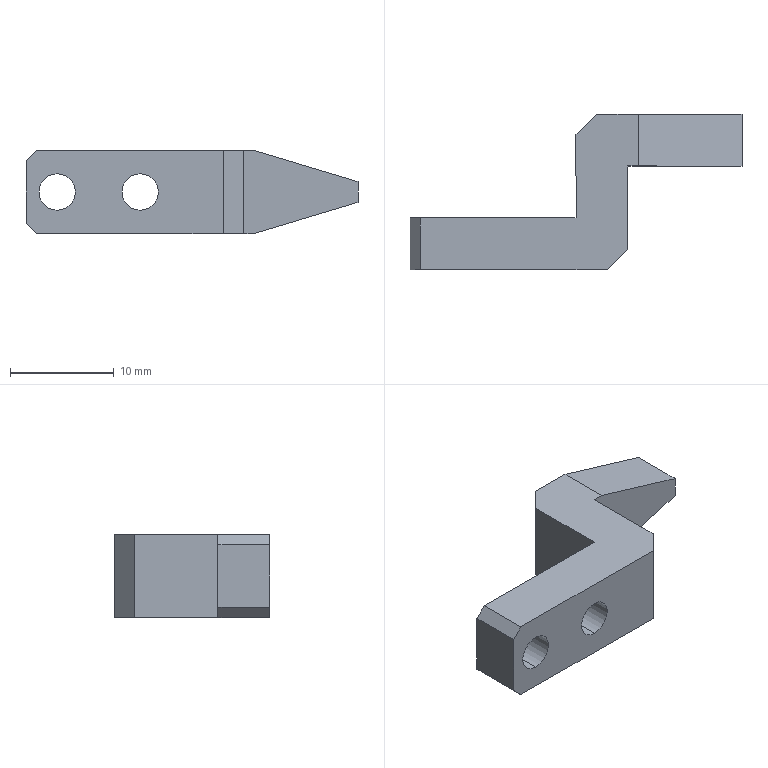Part | SolidWorks | features Chamfer 4, Extrusion 1, HoleWzd 1, ICE 1 | 1 solid | 20 faces | box 32 x 15 x 8 mm | volume 1397 mm3 | plane 16 | cylinder 4 | commonest cylinder face diameters 3.5 x4
STEP:
#1=CARTESIAN_POINT('',(-13.,-7.5,-1.75));
#2=VERTEX_POINT('',#1);
#3=CARTESIAN_POINT('',(-13.,-7.5,1.75));
#4=VERTEX_POINT('',#3);
#5=CARTESIAN_POINT('',(-13.,-7.5,0.));
#6=DIRECTION('',(0.,1.,0.));
#7=DIRECTION('',(0.,0.,1.));
#8=AXIS2_PLACEMENT_3D('',#5,#6,#7);
#9=CIRCLE('',#8,1.75);
#10=EDGE_CURVE('',#2,#4,#9,.T.);
#11=ORIENTED_EDGE('',*,*,#10,.F.);
#12=CARTESIAN_POINT('',(-13.,-2.5,-1.75));
#13=VERTEX_POINT('',#12);
#14=CARTESIAN_POINT('',(-13.,-2.5,-1.75));
#15=DIRECTION('',(0.,1.,0.));
#16=VECTOR('',#15,1000.);
#17=LINE('',#14,#16);
#18=EDGE_CURVE('',#2,#13,#17,.T.);
#19=ORIENTED_EDGE('',*,*,#18,.T.);
#20=CARTESIAN_POINT('',(-13.,-2.5,1.75));
#21=VERTEX_POINT('',#20);
#22=CARTESIAN_POINT('',(-13.,-2.5,0.));
#23=DIRECTION('',(0.,1.,0.));
#24=DIRECTION('',(0.,0.,1.));
#25=AXIS2_PLACEMENT_3D('',#22,#23,#24);
#26=CIRCLE('',#25,1.75);
#27=EDGE_CURVE('',#13,#21,#26,.T.);
#28=ORIENTED_EDGE('',*,*,#27,.T.);
#29=CARTESIAN_POINT('',(-13.,-2.5,1.75));
#30=DIRECTION('',(0.,1.,0.));
#31=VECTOR('',#30,1000.);
#32=LINE('',#29,#31);
#33=EDGE_CURVE('',#4,#21,#32,.T.);
#34=ORIENTED_EDGE('',*,*,#33,.F.);
#35=EDGE_LOOP('',(#11,#19,#28,#34));
#36=FACE_OUTER_BOUND('',#35,.T.);
#37=CARTESIAN_POINT('',(-13.,-2.5,0.));
#38=DIRECTION('',(0.,1.,0.));
#39=DIRECTION('',(0.,0.,1.));
#40=AXIS2_PLACEMENT_3D('',#37,#38,#39);
#41=CYLINDRICAL_SURFACE('',#40,1.75);
#42=ADVANCED_FACE('',(#36),#41,.F.);
#43=CARTESIAN_POINT('',(-5.,-7.5,-1.75));
#44=VERTEX_POINT('',#43);
#45=CARTESIAN_POINT('',(-5.,-7.5,1.75));
#46=VERTEX_POINT('',#45);
#47=CARTESIAN_POINT('',(-5.,-7.5,0.));
#48=DIRECTION('',(0.,1.,0.));
#49=DIRECTION('',(0.,0.,1.));
#50=AXIS2_PLACEMENT_3D('',#47,#48,#49);
#51=CIRCLE('',#50,1.75);
#52=EDGE_CURVE('',#44,#46,#51,.T.);
#53=ORIENTED_EDGE('',*,*,#52,.F.);
#54=CARTESIAN_POINT('',(-5.,-2.5,-1.75));
#55=VERTEX_POINT('',#54);
#56=CARTESIAN_POINT('',(-5.,-2.5,-1.75));
#57=DIRECTION('',(0.,1.,0.));
#58=VECTOR('',#57,1000.);
#59=LINE('',#56,#58);
#60=EDGE_CURVE('',#44,#55,#59,.T.);
#61=ORIENTED_EDGE('',*,*,#60,.T.);
#62=CARTESIAN_POINT('',(-5.,-2.5,1.75));
#63=VERTEX_POINT('',#62);
#64=CARTESIAN_POINT('',(-5.,-2.5,0.));
#65=DIRECTION('',(0.,1.,0.));
#66=DIRECTION('',(0.,0.,1.));
#67=AXIS2_PLACEMENT_3D('',#64,#65,#66);
#68=CIRCLE('',#67,1.75);
#69=EDGE_CURVE('',#55,#63,#68,.T.);
#70=ORIENTED_EDGE('',*,*,#69,.T.);
#71=CARTESIAN_POINT('',(-5.,-2.5,1.75));
#72=DIRECTION('',(0.,1.,0.));
#73=VECTOR('',#72,1000.);
#74=LINE('',#71,#73);
#75=EDGE_CURVE('',#46,#63,#74,.T.);
#76=ORIENTED_EDGE('',*,*,#75,.F.);
#77=EDGE_LOOP('',(#53,#61,#70,#76));
#78=FACE_OUTER_BOUND('',#77,.T.);
#79=CARTESIAN_POINT('',(-5.,-2.5,0.));
#80=DIRECTION('',(0.,1.,0.));
#81=DIRECTION('',(0.,0.,1.));
#82=AXIS2_PLACEMENT_3D('',#79,#80,#81);
#83=CYLINDRICAL_SURFACE('',#82,1.75);
#84=ADVANCED_FACE('',(#78),#83,.F.);
#85=CARTESIAN_POINT('',(16.,2.5,-1.));
#86=VERTEX_POINT('',#85);
#87=CARTESIAN_POINT('',(16.,2.5,1.));
#88=VERTEX_POINT('',#87);
#89=CARTESIAN_POINT('',(16.,2.5,-4.));
#90=DIRECTION('',(0.,0.,1.));
#91=VECTOR('',#90,1000.);
#92=LINE('',#89,#91);
#93=EDGE_CURVE('',#86,#88,#92,.T.);
#94=ORIENTED_EDGE('',*,*,#93,.F.);
#95=CARTESIAN_POINT('',(16.,7.5,-1.));
#96=VERTEX_POINT('',#95);
#97=CARTESIAN_POINT('',(16.,7.5,-1.));
#98=DIRECTION('',(0.,1.,0.));
#99=VECTOR('',#98,1000.);
#100=LINE('',#97,#99);
#101=EDGE_CURVE('',#86,#96,#100,.T.);
#102=ORIENTED_EDGE('',*,*,#101,.T.);
#103=CARTESIAN_POINT('',(16.,7.5,1.));
#104=VERTEX_POINT('',#103);
#105=CARTESIAN_POINT('',(16.,7.5,4.));
#106=DIRECTION('',(0.,0.,-1.));
#107=VECTOR('',#106,1000.);
#108=LINE('',#105,#107);
#109=EDGE_CURVE('',#104,#96,#108,.T.);
#110=ORIENTED_EDGE('',*,*,#109,.F.);
#111=CARTESIAN_POINT('',(16.,2.5,1.));
#112=DIRECTION('',(0.,-1.,0.));
#113=VECTOR('',#112,1000.);
#114=LINE('',#111,#113);
#115=EDGE_CURVE('',#104,#88,#114,.T.);
#116=ORIENTED_EDGE('',*,*,#115,.T.);
#117=EDGE_LOOP('',(#94,#102,#110,#116));
#118=FACE_OUTER_BOUND('',#117,.T.);
#119=CARTESIAN_POINT('',(16.,7.5,4.));
#120=DIRECTION('',(-1.,0.,0.));
#121=DIRECTION('',(0.,-1.,0.));
#122=AXIS2_PLACEMENT_3D('',#119,#120,#121);
#123=PLANE('',#122);
#124=ADVANCED_FACE('',(#118),#123,.F.);
#125=ORIENTED_EDGE('',*,*,#109,.T.);
#126=CARTESIAN_POINT('',(6.,7.5,-4.));
#127=VERTEX_POINT('',#126);
#128=CARTESIAN_POINT('',(16.,7.5,-1.));
#129=DIRECTION('',(-0.9578,0.,-0.2873));
#130=VECTOR('',#129,1000.);
#131=LINE('',#128,#130);
#132=EDGE_CURVE('',#96,#127,#131,.T.);
#133=ORIENTED_EDGE('',*,*,#132,.T.);
#134=CARTESIAN_POINT('',(2.,7.5,-4.));
#135=VERTEX_POINT('',#134);
#136=CARTESIAN_POINT('',(-16.,7.5,-4.));
#137=DIRECTION('',(-1.,0.,0.));
#138=VECTOR('',#137,1000.);
#139=LINE('',#136,#138);
#140=EDGE_CURVE('',#127,#135,#139,.T.);
#141=ORIENTED_EDGE('',*,*,#140,.T.);
#142=CARTESIAN_POINT('',(2.,7.5,4.));
#143=VERTEX_POINT('',#142);
#144=CARTESIAN_POINT('',(2.,7.5,4.));
#145=DIRECTION('',(0.,0.,1.));
#146=VECTOR('',#145,1000.);
#147=LINE('',#144,#146);
#148=EDGE_CURVE('',#135,#143,#147,.T.);
#149=ORIENTED_EDGE('',*,*,#148,.T.);
#150=CARTESIAN_POINT('',(6.,7.5,4.));
#151=VERTEX_POINT('',#150);
#152=CARTESIAN_POINT('',(-16.,7.5,4.));
#153=DIRECTION('',(-1.,0.,0.));
#154=VECTOR('',#153,1000.);
#155=LINE('',#152,#154);
#156=EDGE_CURVE('',#151,#143,#155,.T.);
#157=ORIENTED_EDGE('',*,*,#156,.F.);
#158=CARTESIAN_POINT('',(6.,7.5,4.));
#159=DIRECTION('',(0.9578,0.,-0.2873));
#160=VECTOR('',#159,1000.);
#161=LINE('',#158,#160);
#162=EDGE_CURVE('',#151,#104,#161,.T.);
#163=ORIENTED_EDGE('',*,*,#162,.T.);
#164=EDGE_LOOP('',(#125,#133,#141,#149,#157,#163));
#165=FACE_OUTER_BOUND('',#164,.T.);
#166=CARTESIAN_POINT('',(-16.,7.5,4.));
#167=DIRECTION('',(0.,-1.,0.));
#168=DIRECTION('',(0.,0.,-1.));
#169=AXIS2_PLACEMENT_3D('',#166,#167,#168);
#170=PLANE('',#169);
#171=ADVANCED_FACE('',(#165),#170,.F.);
#172=CARTESIAN_POINT('',(-16.,-2.5,-3.));
#173=VERTEX_POINT('',#172);
#174=CARTESIAN_POINT('',(-16.,-2.5,3.));
#175=VERTEX_POINT('',#174);
#176=CARTESIAN_POINT('',(-16.,-2.5,-4.));
#177=DIRECTION('',(0.,0.,1.));
#178=VECTOR('',#177,1000.);
#179=LINE('',#176,#178);
#180=EDGE_CURVE('',#173,#175,#179,.T.);
#181=ORIENTED_EDGE('',*,*,#180,.F.);
#182=CARTESIAN_POINT('',(-16.,-7.5,-3.));
#183=VERTEX_POINT('',#182);
#184=CARTESIAN_POINT('',(-16.,7.5,-3.));
#185=DIRECTION('',(0.,-1.,0.));
#186=VECTOR('',#185,1000.);
#187=LINE('',#184,#186);
#188=EDGE_CURVE('',#173,#183,#187,.T.);
#189=ORIENTED_EDGE('',*,*,#188,.T.);
#190=CARTESIAN_POINT('',(-16.,-7.5,3.));
#191=VERTEX_POINT('',#190);
#192=CARTESIAN_POINT('',(-16.,-7.5,4.));
#193=DIRECTION('',(0.,0.,-1.));
#194=VECTOR('',#193,1000.);
#195=LINE('',#192,#194);
#196=EDGE_CURVE('',#191,#183,#195,.T.);
#197=ORIENTED_EDGE('',*,*,#196,.F.);
#198=CARTESIAN_POINT('',(-16.,-2.5,3.));
#199=DIRECTION('',(0.,1.,0.));
#200=VECTOR('',#199,1000.);
#201=LINE('',#198,#200);
#202=EDGE_CURVE('',#191,#175,#201,.T.);
#203=ORIENTED_EDGE('',*,*,#202,.T.);
#204=EDGE_LOOP('',(#181,#189,#197,#203));
#205=FACE_OUTER_BOUND('',#204,.T.);
#206=CARTESIAN_POINT('',(-16.,7.5,4.));
#207=DIRECTION('',(1.,0.,0.));
#208=DIRECTION('',(0.,1.,0.));
#209=AXIS2_PLACEMENT_3D('',#206,#207,#208);
#210=PLANE('',#209);
#211=ADVANCED_FACE('',(#205),#210,.F.);
#212=CARTESIAN_POINT('',(-13.,-7.5,0.));
#213=DIRECTION('',(0.,1.,0.));
#214=DIRECTION('',(0.,0.,1.));
#215=AXIS2_PLACEMENT_3D('',#212,#213,#214);
#216=CIRCLE('',#215,1.75);
#217=EDGE_CURVE('',#4,#2,#216,.T.);
#218=ORIENTED_EDGE('',*,*,#217,.T.);
#219=ORIENTED_EDGE('',*,*,#10,.T.);
#220=EDGE_LOOP('',(#218,#219));
#221=FACE_BOUND('',#220,.T.);
#222=CARTESIAN_POINT('',(-5.,-7.5,0.));
#223=DIRECTION('',(0.,1.,0.));
#224=DIRECTION('',(0.,0.,1.));
#225=AXIS2_PLACEMENT_3D('',#222,#223,#224);
#226=CIRCLE('',#225,1.75);
#227=EDGE_CURVE('',#46,#44,#226,.T.);
#228=ORIENTED_EDGE('',*,*,#227,.T.);
#229=ORIENTED_EDGE('',*,*,#52,.T.);
#230=EDGE_LOOP('',(#228,#229));
#231=FACE_BOUND('',#230,.T.);
#232=CARTESIAN_POINT('',(-15.,-7.5,-4.));
#233=VERTEX_POINT('',#232);
#234=CARTESIAN_POINT('',(3.,-7.5,-4.));
#235=VERTEX_POINT('',#234);
#236=CARTESIAN_POINT('',(-16.,-7.5,-4.));
#237=DIRECTION('',(1.,0.,0.));
#238=VECTOR('',#237,1000.);
#239=LINE('',#236,#238);
#240=EDGE_CURVE('',#233,#235,#239,.T.);
#241=ORIENTED_EDGE('',*,*,#240,.T.);
#242=CARTESIAN_POINT('',(3.,-7.5,4.));
#243=VERTEX_POINT('',#242);
#244=CARTESIAN_POINT('',(3.,-7.5,4.));
#245=DIRECTION('',(0.,0.,1.));
#246=VECTOR('',#245,1000.);
#247=LINE('',#244,#246);
#248=EDGE_CURVE('',#235,#243,#247,.T.);
#249=ORIENTED_EDGE('',*,*,#248,.T.);
#250=CARTESIAN_POINT('',(-15.,-7.5,4.));
#251=VERTEX_POINT('',#250);
#252=CARTESIAN_POINT('',(-16.,-7.5,4.));
#253=DIRECTION('',(1.,0.,0.));
#254=VECTOR('',#253,1000.);
#255=LINE('',#252,#254);
#256=EDGE_CURVE('',#251,#243,#255,.T.);
#257=ORIENTED_EDGE('',*,*,#256,.F.);
#258=CARTESIAN_POINT('',(-15.,-7.5,4.));
#259=DIRECTION('',(-0.7071,0.,-0.7071));
#260=VECTOR('',#259,1000.);
#261=LINE('',#258,#260);
#262=EDGE_CURVE('',#251,#191,#261,.T.);
#263=ORIENTED_EDGE('',*,*,#262,.T.);
#264=ORIENTED_EDGE('',*,*,#196,.T.);
#265=CARTESIAN_POINT('',(-16.,-7.5,-3.));
#266=DIRECTION('',(0.7071,0.,-0.7071));
#267=VECTOR('',#266,1000.);
#268=LINE('',#265,#267);
#269=EDGE_CURVE('',#183,#233,#268,.T.);
#270=ORIENTED_EDGE('',*,*,#269,.T.);
#271=EDGE_LOOP('',(#241,#249,#257,#263,#264,#270));
#272=FACE_OUTER_BOUND('',#271,.T.);
#273=CARTESIAN_POINT('',(-16.,-7.5,4.));
#274=DIRECTION('',(0.,1.,0.));
#275=DIRECTION('',(0.,0.,1.));
#276=AXIS2_PLACEMENT_3D('',#273,#274,#275);
#277=PLANE('',#276);
#278=ADVANCED_FACE('',(#221,#231,#272),#277,.F.);
#279=CARTESIAN_POINT('',(6.,2.5,4.));
#280=VERTEX_POINT('',#279);
#281=CARTESIAN_POINT('',(5.,2.5,4.));
#282=VERTEX_POINT('',#281);
#283=CARTESIAN_POINT('',(16.,2.5,4.));
#284=DIRECTION('',(-1.,0.,0.));
#285=VECTOR('',#284,1000.);
#286=LINE('',#283,#285);
#287=EDGE_CURVE('',#280,#282,#286,.T.);
#288=ORIENTED_EDGE('',*,*,#287,.F.);
#289=CARTESIAN_POINT('',(6.,7.5,4.));
#290=DIRECTION('',(0.,1.,0.));
#291=VECTOR('',#290,1000.);
#292=LINE('',#289,#291);
#293=EDGE_CURVE('',#280,#151,#292,.T.);
#294=ORIENTED_EDGE('',*,*,#293,.T.);
#295=ORIENTED_EDGE('',*,*,#156,.T.);
#296=CARTESIAN_POINT('',(0.,5.5,4.));
#297=VERTEX_POINT('',#296);
#298=CARTESIAN_POINT('',(-2.75,2.75,4.));
#299=DIRECTION('',(-0.7071,-0.7071,0.));
#300=VECTOR('',#299,1000.);
#301=LINE('',#298,#300);
#302=EDGE_CURVE('',#143,#297,#301,.T.);
#303=ORIENTED_EDGE('',*,*,#302,.T.);
#304=CARTESIAN_POINT('',(0.,-2.5,4.));
#305=VERTEX_POINT('',#304);
#306=CARTESIAN_POINT('',(0.,7.5,4.));
#307=DIRECTION('',(0.,1.,0.));
#308=VECTOR('',#307,1000.);
#309=LINE('',#306,#308);
#310=EDGE_CURVE('',#305,#297,#309,.T.);
#311=ORIENTED_EDGE('',*,*,#310,.F.);
#312=CARTESIAN_POINT('',(-15.,-2.5,4.));
#313=VERTEX_POINT('',#312);
#314=CARTESIAN_POINT('',(-16.,-2.5,4.));
#315=DIRECTION('',(1.,0.,0.));
#316=VECTOR('',#315,1000.);
#317=LINE('',#314,#316);
#318=EDGE_CURVE('',#313,#305,#317,.T.);
#319=ORIENTED_EDGE('',*,*,#318,.F.);
#320=CARTESIAN_POINT('',(-15.,-7.5,4.));
#321=DIRECTION('',(0.,-1.,0.));
#322=VECTOR('',#321,1000.);
#323=LINE('',#320,#322);
#324=EDGE_CURVE('',#313,#251,#323,.T.);
#325=ORIENTED_EDGE('',*,*,#324,.T.);
#326=ORIENTED_EDGE('',*,*,#256,.T.);
#327=CARTESIAN_POINT('',(5.,-5.5,4.));
#328=VERTEX_POINT('',#327);
#329=CARTESIAN_POINT('',(5.25,-5.25,4.));
#330=DIRECTION('',(0.7071,0.7071,0.));
#331=VECTOR('',#330,1000.);
#332=LINE('',#329,#331);
#333=EDGE_CURVE('',#243,#328,#332,.T.);
#334=ORIENTED_EDGE('',*,*,#333,.T.);
#335=CARTESIAN_POINT('',(5.,-7.5,4.));
#336=DIRECTION('',(0.,-1.,0.));
#337=VECTOR('',#336,1000.);
#338=LINE('',#335,#337);
#339=EDGE_CURVE('',#282,#328,#338,.T.);
#340=ORIENTED_EDGE('',*,*,#339,.F.);
#341=EDGE_LOOP('',(#288,#294,#295,#303,#311,#319,#325,#326,#334,#340));
#342=FACE_OUTER_BOUND('',#341,.T.);
#343=CARTESIAN_POINT('',(0.,0.,4.));
#344=DIRECTION('',(0.,0.,1.));
#345=DIRECTION('',(1.,0.,0.));
#346=AXIS2_PLACEMENT_3D('',#343,#344,#345);
#347=PLANE('',#346);
#348=ADVANCED_FACE('',(#342),#347,.T.);
#349=ORIENTED_EDGE('',*,*,#140,.F.);
#350=CARTESIAN_POINT('',(6.,2.5,-4.));
#351=VERTEX_POINT('',#350);
#352=CARTESIAN_POINT('',(6.,0.,-4.));
#353=DIRECTION('',(0.,-1.,0.));
#354=VECTOR('',#353,1000.);
#355=LINE('',#352,#354);
#356=EDGE_CURVE('',#127,#351,#355,.T.);
#357=ORIENTED_EDGE('',*,*,#356,.T.);
#358=CARTESIAN_POINT('',(5.,2.5,-4.));
#359=VERTEX_POINT('',#358);
#360=CARTESIAN_POINT('',(16.,2.5,-4.));
#361=DIRECTION('',(-1.,0.,0.));
#362=VECTOR('',#361,1000.);
#363=LINE('',#360,#362);
#364=EDGE_CURVE('',#351,#359,#363,.T.);
#365=ORIENTED_EDGE('',*,*,#364,.T.);
#366=CARTESIAN_POINT('',(5.,-5.5,-4.));
#367=VERTEX_POINT('',#366);
#368=CARTESIAN_POINT('',(5.,-7.5,-4.));
#369=DIRECTION('',(0.,-1.,0.));
#370=VECTOR('',#369,1000.);
#371=LINE('',#368,#370);
#372=EDGE_CURVE('',#359,#367,#371,.T.);
#373=ORIENTED_EDGE('',*,*,#372,.T.);
#374=CARTESIAN_POINT('',(3.,-7.5,-4.));
#375=DIRECTION('',(-0.7071,-0.7071,0.));
#376=VECTOR('',#375,1000.);
#377=LINE('',#374,#376);
#378=EDGE_CURVE('',#367,#235,#377,.T.);
#379=ORIENTED_EDGE('',*,*,#378,.T.);
#380=ORIENTED_EDGE('',*,*,#240,.F.);
#381=CARTESIAN_POINT('',(-15.,-2.5,-4.));
#382=VERTEX_POINT('',#381);
#383=CARTESIAN_POINT('',(-15.,0.,-4.));
#384=DIRECTION('',(0.,1.,0.));
#385=VECTOR('',#384,1000.);
#386=LINE('',#383,#385);
#387=EDGE_CURVE('',#233,#382,#386,.T.);
#388=ORIENTED_EDGE('',*,*,#387,.T.);
#389=CARTESIAN_POINT('',(0.,-2.5,-4.));
#390=VERTEX_POINT('',#389);
#391=CARTESIAN_POINT('',(-16.,-2.5,-4.));
#392=DIRECTION('',(1.,0.,0.));
#393=VECTOR('',#392,1000.);
#394=LINE('',#391,#393);
#395=EDGE_CURVE('',#382,#390,#394,.T.);
#396=ORIENTED_EDGE('',*,*,#395,.T.);
#397=CARTESIAN_POINT('',(0.,5.5,-4.));
#398=VERTEX_POINT('',#397);
#399=CARTESIAN_POINT('',(0.,7.5,-4.));
#400=DIRECTION('',(0.,1.,0.));
#401=VECTOR('',#400,1000.);
#402=LINE('',#399,#401);
#403=EDGE_CURVE('',#390,#398,#402,.T.);
#404=ORIENTED_EDGE('',*,*,#403,.T.);
#405=CARTESIAN_POINT('',(2.,7.5,-4.));
#406=DIRECTION('',(0.7071,0.7071,0.));
#407=VECTOR('',#406,1000.);
#408=LINE('',#405,#407);
#409=EDGE_CURVE('',#398,#135,#408,.T.);
#410=ORIENTED_EDGE('',*,*,#409,.T.);
#411=EDGE_LOOP('',(#349,#357,#365,#373,#379,#380,#388,#396,#404,#410));
#412=FACE_OUTER_BOUND('',#411,.T.);
#413=CARTESIAN_POINT('',(0.,0.,-4.));
#414=DIRECTION('',(0.,0.,1.));
#415=DIRECTION('',(1.,0.,0.));
#416=AXIS2_PLACEMENT_3D('',#413,#414,#415);
#417=PLANE('',#416);
#418=ADVANCED_FACE('',(#412),#417,.F.);
#419=ORIENTED_EDGE('',*,*,#310,.T.);
#420=CARTESIAN_POINT('',(0.,5.5,-4.));
#421=DIRECTION('',(0.,0.,-1.));
#422=VECTOR('',#421,1000.);
#423=LINE('',#420,#422);
#424=EDGE_CURVE('',#297,#398,#423,.T.);
#425=ORIENTED_EDGE('',*,*,#424,.T.);
#426=ORIENTED_EDGE('',*,*,#403,.F.);
#427=CARTESIAN_POINT('',(0.,-2.5,-4.));
#428=DIRECTION('',(0.,0.,1.));
#429=VECTOR('',#428,1000.);
#430=LINE('',#427,#429);
#431=EDGE_CURVE('',#390,#305,#430,.T.);
#432=ORIENTED_EDGE('',*,*,#431,.T.);
#433=EDGE_LOOP('',(#419,#425,#426,#432));
#434=FACE_OUTER_BOUND('',#433,.T.);
#435=CARTESIAN_POINT('',(0.,7.5,-4.));
#436=DIRECTION('',(1.,0.,0.));
#437=DIRECTION('',(0.,1.,0.));
#438=AXIS2_PLACEMENT_3D('',#435,#436,#437);
#439=PLANE('',#438);
#440=ADVANCED_FACE('',(#434),#439,.F.);
#441=CARTESIAN_POINT('',(-13.,-2.5,0.));
#442=DIRECTION('',(0.,1.,0.));
#443=DIRECTION('',(0.,0.,1.));
#444=AXIS2_PLACEMENT_3D('',#441,#442,#443);
#445=CIRCLE('',#444,1.75);
#446=EDGE_CURVE('',#21,#13,#445,.T.);
#447=ORIENTED_EDGE('',*,*,#446,.F.);
#448=ORIENTED_EDGE('',*,*,#27,.F.);
#449=EDGE_LOOP('',(#447,#448));
#450=FACE_BOUND('',#449,.T.);
#451=CARTESIAN_POINT('',(-5.,-2.5,0.));
#452=DIRECTION('',(0.,1.,0.));
#453=DIRECTION('',(0.,0.,1.));
#454=AXIS2_PLACEMENT_3D('',#451,#452,#453);
#455=CIRCLE('',#454,1.75);
#456=EDGE_CURVE('',#63,#55,#455,.T.);
#457=ORIENTED_EDGE('',*,*,#456,.F.);
#458=ORIENTED_EDGE('',*,*,#69,.F.);
#459=EDGE_LOOP('',(#457,#458));
#460=FACE_BOUND('',#459,.T.);
#461=ORIENTED_EDGE('',*,*,#395,.F.);
#462=CARTESIAN_POINT('',(-16.,-2.5,-3.));
#463=DIRECTION('',(-0.7071,0.,0.7071));
#464=VECTOR('',#463,1000.);
#465=LINE('',#462,#464);
#466=EDGE_CURVE('',#382,#173,#465,.T.);
#467=ORIENTED_EDGE('',*,*,#466,.T.);
#468=ORIENTED_EDGE('',*,*,#180,.T.);
#469=CARTESIAN_POINT('',(-15.,-2.5,4.));
#470=DIRECTION('',(0.7071,0.,0.7071));
#471=VECTOR('',#470,1000.);
#472=LINE('',#469,#471);
#473=EDGE_CURVE('',#175,#313,#472,.T.);
#474=ORIENTED_EDGE('',*,*,#473,.T.);
#475=ORIENTED_EDGE('',*,*,#318,.T.);
#476=ORIENTED_EDGE('',*,*,#431,.F.);
#477=EDGE_LOOP('',(#461,#467,#468,#474,#475,#476));
#478=FACE_OUTER_BOUND('',#477,.T.);
#479=CARTESIAN_POINT('',(-16.,-2.5,-4.));
#480=DIRECTION('',(0.,-1.,0.));
#481=DIRECTION('',(0.,0.,-1.));
#482=AXIS2_PLACEMENT_3D('',#479,#480,#481);
#483=PLANE('',#482);
#484=ADVANCED_FACE('',(#450,#460,#478),#483,.F.);
#485=ORIENTED_EDGE('',*,*,#339,.T.);
#486=CARTESIAN_POINT('',(5.,-5.5,-4.));
#487=DIRECTION('',(0.,0.,-1.));
#488=VECTOR('',#487,1000.);
#489=LINE('',#486,#488);
#490=EDGE_CURVE('',#328,#367,#489,.T.);
#491=ORIENTED_EDGE('',*,*,#490,.T.);
#492=ORIENTED_EDGE('',*,*,#372,.F.);
#493=CARTESIAN_POINT('',(5.,2.5,-4.));
#494=DIRECTION('',(0.,0.,1.));
#495=VECTOR('',#494,1000.);
#496=LINE('',#493,#495);
#497=EDGE_CURVE('',#359,#282,#496,.T.);
#498=ORIENTED_EDGE('',*,*,#497,.T.);
#499=EDGE_LOOP('',(#485,#491,#492,#498));
#500=FACE_OUTER_BOUND('',#499,.T.);
#501=CARTESIAN_POINT('',(5.,-7.5,-4.));
#502=DIRECTION('',(-1.,0.,0.));
#503=DIRECTION('',(0.,0.,1.));
#504=AXIS2_PLACEMENT_3D('',#501,#502,#503);
#505=PLANE('',#504);
#506=ADVANCED_FACE('',(#500),#505,.F.);
#507=ORIENTED_EDGE('',*,*,#364,.F.);
#508=CARTESIAN_POINT('',(16.,2.5,-1.));
#509=DIRECTION('',(0.9578,0.,0.2873));
#510=VECTOR('',#509,1000.);
#511=LINE('',#508,#510);
#512=EDGE_CURVE('',#351,#86,#511,.T.);
#513=ORIENTED_EDGE('',*,*,#512,.T.);
#514=ORIENTED_EDGE('',*,*,#93,.T.);
#515=CARTESIAN_POINT('',(6.,2.5,4.));
#516=DIRECTION('',(-0.9578,0.,0.2873));
#517=VECTOR('',#516,1000.);
#518=LINE('',#515,#517);
#519=EDGE_CURVE('',#88,#280,#518,.T.);
#520=ORIENTED_EDGE('',*,*,#519,.T.);
#521=ORIENTED_EDGE('',*,*,#287,.T.);
#522=ORIENTED_EDGE('',*,*,#497,.F.);
#523=EDGE_LOOP('',(#507,#513,#514,#520,#521,#522));
#524=FACE_OUTER_BOUND('',#523,.T.);
#525=CARTESIAN_POINT('',(16.,2.5,-4.));
#526=DIRECTION('',(0.,1.,0.));
#527=DIRECTION('',(-1.,0.,0.));
#528=AXIS2_PLACEMENT_3D('',#525,#526,#527);
#529=PLANE('',#528);
#530=ADVANCED_FACE('',(#524),#529,.F.);
#531=ORIENTED_EDGE('',*,*,#466,.F.);
#532=ORIENTED_EDGE('',*,*,#387,.F.);
#533=ORIENTED_EDGE('',*,*,#269,.F.);
#534=ORIENTED_EDGE('',*,*,#188,.F.);
#535=EDGE_LOOP('',(#531,#532,#533,#534));
#536=FACE_OUTER_BOUND('',#535,.T.);
#537=CARTESIAN_POINT('',(-16.,7.5,-3.));
#538=DIRECTION('',(0.7071,0.,0.7071));
#539=DIRECTION('',(0.,-1.,0.));
#540=AXIS2_PLACEMENT_3D('',#537,#538,#539);
#541=PLANE('',#540);
#542=ADVANCED_FACE('',(#536),#541,.F.);
#543=ORIENTED_EDGE('',*,*,#473,.F.);
#544=ORIENTED_EDGE('',*,*,#202,.F.);
#545=ORIENTED_EDGE('',*,*,#262,.F.);
#546=ORIENTED_EDGE('',*,*,#324,.F.);
#547=EDGE_LOOP('',(#543,#544,#545,#546));
#548=FACE_OUTER_BOUND('',#547,.T.);
#549=CARTESIAN_POINT('',(-15.,0.,4.));
#550=DIRECTION('',(-0.7071,0.,0.7071));
#551=DIRECTION('',(0.,1.,0.));
#552=AXIS2_PLACEMENT_3D('',#549,#550,#551);
#553=PLANE('',#552);
#554=ADVANCED_FACE('',(#548),#553,.T.);
#555=ORIENTED_EDGE('',*,*,#378,.F.);
#556=ORIENTED_EDGE('',*,*,#490,.F.);
#557=ORIENTED_EDGE('',*,*,#333,.F.);
#558=ORIENTED_EDGE('',*,*,#248,.F.);
#559=EDGE_LOOP('',(#555,#556,#557,#558));
#560=FACE_OUTER_BOUND('',#559,.T.);
#561=CARTESIAN_POINT('',(3.,-7.5,4.));
#562=DIRECTION('',(-0.7071,0.7071,0.));
#563=DIRECTION('',(0.,0.,1.));
#564=AXIS2_PLACEMENT_3D('',#561,#562,#563);
#565=PLANE('',#564);
#566=ADVANCED_FACE('',(#560),#565,.F.);
#567=ORIENTED_EDGE('',*,*,#409,.F.);
#568=ORIENTED_EDGE('',*,*,#424,.F.);
#569=ORIENTED_EDGE('',*,*,#302,.F.);
#570=ORIENTED_EDGE('',*,*,#148,.F.);
#571=EDGE_LOOP('',(#567,#568,#569,#570));
#572=FACE_OUTER_BOUND('',#571,.T.);
#573=CARTESIAN_POINT('',(2.,7.5,4.));
#574=DIRECTION('',(0.7071,-0.7071,0.));
#575=DIRECTION('',(0.,0.,1.));
#576=AXIS2_PLACEMENT_3D('',#573,#574,#575);
#577=PLANE('',#576);
#578=ADVANCED_FACE('',(#572),#577,.F.);
#579=ORIENTED_EDGE('',*,*,#60,.F.);
#580=ORIENTED_EDGE('',*,*,#227,.F.);
#581=ORIENTED_EDGE('',*,*,#75,.T.);
#582=ORIENTED_EDGE('',*,*,#456,.T.);
#583=EDGE_LOOP('',(#579,#580,#581,#582));
#584=FACE_OUTER_BOUND('',#583,.T.);
#585=CARTESIAN_POINT('',(-5.,-2.5,0.));
#586=DIRECTION('',(0.,1.,0.));
#587=DIRECTION('',(0.,0.,1.));
#588=AXIS2_PLACEMENT_3D('',#585,#586,#587);
#589=CYLINDRICAL_SURFACE('',#588,1.75);
#590=ADVANCED_FACE('',(#584),#589,.F.);
#591=ORIENTED_EDGE('',*,*,#18,.F.);
#592=ORIENTED_EDGE('',*,*,#217,.F.);
#593=ORIENTED_EDGE('',*,*,#33,.T.);
#594=ORIENTED_EDGE('',*,*,#446,.T.);
#595=EDGE_LOOP('',(#591,#592,#593,#594));
#596=FACE_OUTER_BOUND('',#595,.T.);
#597=CARTESIAN_POINT('',(-13.,-2.5,0.));
#598=DIRECTION('',(0.,1.,0.));
#599=DIRECTION('',(0.,0.,1.));
#600=AXIS2_PLACEMENT_3D('',#597,#598,#599);
#601=CYLINDRICAL_SURFACE('',#600,1.75);
#602=ADVANCED_FACE('',(#596),#601,.F.);
#603=ORIENTED_EDGE('',*,*,#519,.F.);
#604=ORIENTED_EDGE('',*,*,#115,.F.);
#605=ORIENTED_EDGE('',*,*,#162,.F.);
#606=ORIENTED_EDGE('',*,*,#293,.F.);
#607=EDGE_LOOP('',(#603,#604,#605,#606));
#608=FACE_OUTER_BOUND('',#607,.T.);
#609=CARTESIAN_POINT('',(6.,0.,4.));
#610=DIRECTION('',(0.2873,0.,0.9578));
#611=DIRECTION('',(0.,-1.,0.));
#612=AXIS2_PLACEMENT_3D('',#609,#610,#611);
#613=PLANE('',#612);
#614=ADVANCED_FACE('',(#608),#613,.T.);
#615=ORIENTED_EDGE('',*,*,#512,.F.);
#616=ORIENTED_EDGE('',*,*,#356,.F.);
#617=ORIENTED_EDGE('',*,*,#132,.F.);
#618=ORIENTED_EDGE('',*,*,#101,.F.);
#619=EDGE_LOOP('',(#615,#616,#617,#618));
#620=FACE_OUTER_BOUND('',#619,.T.);
#621=CARTESIAN_POINT('',(16.,7.5,-1.));
#622=DIRECTION('',(-0.2873,0.,0.9578));
#623=DIRECTION('',(0.,1.,0.));
#624=AXIS2_PLACEMENT_3D('',#621,#622,#623);
#625=PLANE('',#624);
#626=ADVANCED_FACE('',(#620),#625,.F.);
#627=CLOSED_SHELL('',(#42,#84,#124,#171,#211,#278,#348,#418,#440,#484,#506,#530,#542,#554,#566,#578,#590,#602,#614,#626));
#628=MANIFOLD_SOLID_BREP('',#627);
#629=CARTESIAN_POINT('',(0.,0.,0.));
#630=DIRECTION('',(0.,0.,1.));
#631=DIRECTION('',(1.,0.,0.));
#632=AXIS2_PLACEMENT_3D('',#629,#630,#631);
#633=(LENGTH_UNIT()NAMED_UNIT(*)SI_UNIT(.MILLI.,.METRE.));
#634=UNCERTAINTY_MEASURE_WITH_UNIT(LENGTH_MEASURE(0.00001),#633,'','');
#635=(NAMED_UNIT(*)PLANE_ANGLE_UNIT()SI_UNIT($,.RADIAN.));
#636=(NAMED_UNIT(*)SI_UNIT($,.STERADIAN.)SOLID_ANGLE_UNIT());
#637=(GEOMETRIC_REPRESENTATION_CONTEXT(3)GLOBAL_UNCERTAINTY_ASSIGNED_CONTEXT((#634))GLOBAL_UNIT_ASSIGNED_CONTEXT((#633,#635,#636))REPRESENTATION_CONTEXT('',''));
#638=ADVANCED_BREP_SHAPE_REPRESENTATION('',(#628,#632),#637);